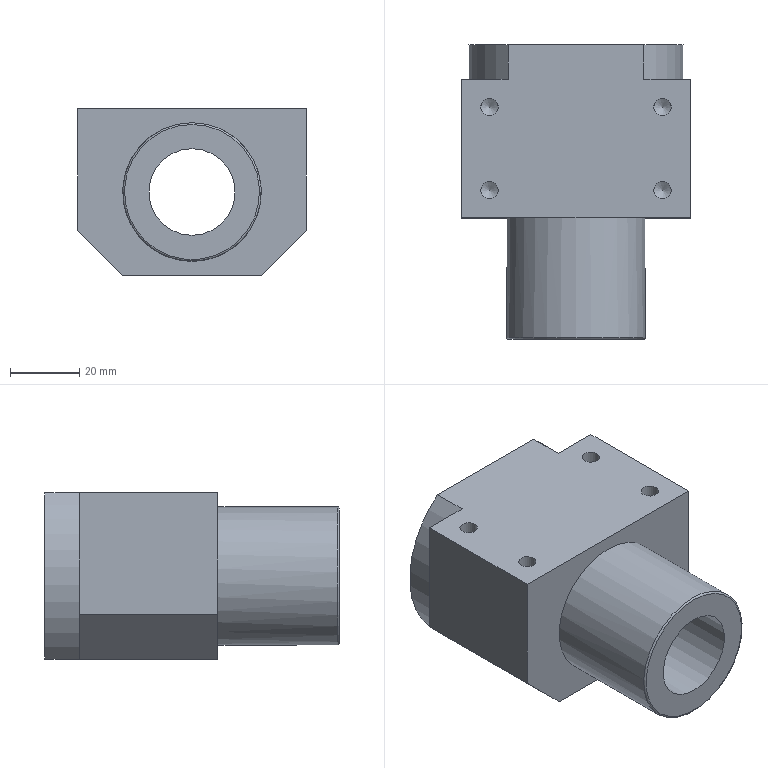Part | STEP file | SFU2510 nut seat_id1010_x_t | 1 solid | 48 faces | box 66 x 85 x 48 mm | volume 143394 mm3 | cylinder 20 | plane 17 | cone 10 | torus 1 | commonest cylinder face diameters 5 x10 6.6 x6 62 x2 25 x1 40 x1